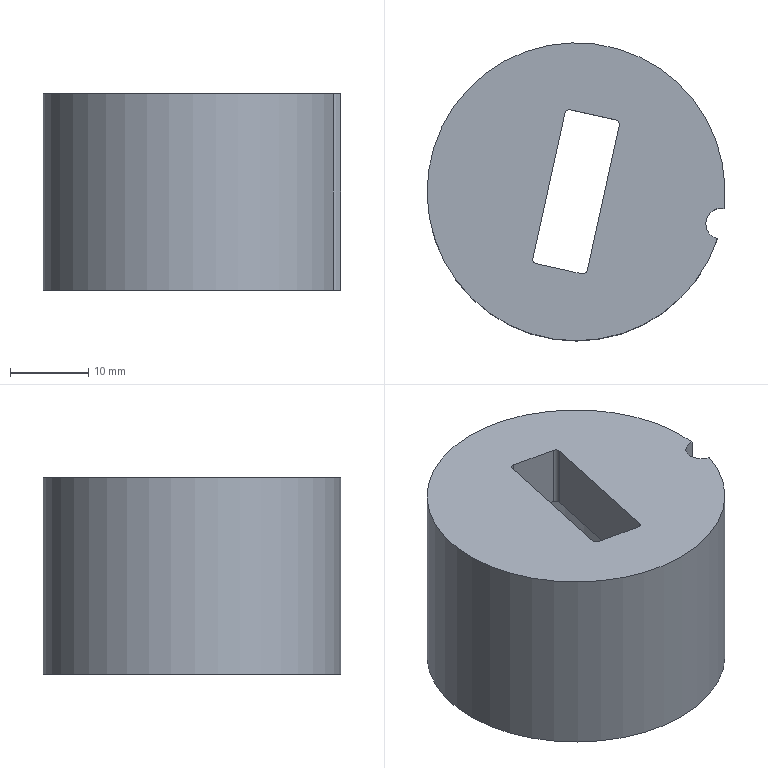Part | NX | features solid 2 | 1 solid | 14 faces | box 38 x 38 x 25 mm | volume 17613 mm3 | cylinder 7 | plane 7 | commonest cylinder face diameters 1.1 x4 4 x1 26.6 x1 38 x1
STEP:
#1=CARTESIAN_POINT('',(36.364,-48.332,31.));
#2=VERTEX_POINT('',#1);
#3=CARTESIAN_POINT('',(36.364,-48.332,56.));
#4=VERTEX_POINT('',#3);
#5=CARTESIAN_POINT('',(36.364,-48.332,43.5));
#6=DIRECTION('',(0.,0.,1.));
#7=VECTOR('',#6,1000.);
#8=LINE('',#5,#7);
#9=EDGE_CURVE('',#2,#4,#8,.T.);
#10=ORIENTED_EDGE('',*,*,#9,.F.);
#11=CARTESIAN_POINT('',(35.507,-52.233,31.));
#12=VERTEX_POINT('',#11);
#13=CARTESIAN_POINT('',(17.482,-46.225,31.));
#14=DIRECTION('',(0.,0.,1.));
#15=DIRECTION('',(0.9767,-0.2148,0.));
#16=AXIS2_PLACEMENT_3D('',#13,#14,#15);
#17=CIRCLE('',#16,19.);
#18=EDGE_CURVE('',#2,#12,#17,.T.);
#19=ORIENTED_EDGE('',*,*,#18,.T.);
#20=CARTESIAN_POINT('',(35.507,-52.233,56.));
#21=VERTEX_POINT('',#20);
#22=CARTESIAN_POINT('',(35.507,-52.233,43.5));
#23=DIRECTION('',(0.,0.,1.));
#24=VECTOR('',#23,1000.);
#25=LINE('',#22,#24);
#26=EDGE_CURVE('',#21,#12,#25,.F.);
#27=ORIENTED_EDGE('',*,*,#26,.F.);
#28=CARTESIAN_POINT('',(17.482,-46.225,56.));
#29=DIRECTION('',(0.,0.,1.));
#30=DIRECTION('',(0.9767,-0.2148,0.));
#31=AXIS2_PLACEMENT_3D('',#28,#29,#30);
#32=CIRCLE('',#31,19.);
#33=EDGE_CURVE('',#4,#21,#32,.T.);
#34=ORIENTED_EDGE('',*,*,#33,.F.);
#35=EDGE_LOOP('',(#10,#19,#27,#34));
#36=FACE_BOUND('',#35,.T.);
#37=CARTESIAN_POINT('',(17.482,-46.225,31.));
#38=DIRECTION('',(0.,0.,1.));
#39=DIRECTION('',(0.9767,-0.2148,0.));
#40=AXIS2_PLACEMENT_3D('',#37,#38,#39);
#41=CYLINDRICAL_SURFACE('',#40,19.);
#42=ADVANCED_FACE('',(#36),#41,.T.);
#43=CARTESIAN_POINT('',(30.471,-49.081,31.));
#44=VERTEX_POINT('',#43);
#45=CARTESIAN_POINT('',(17.482,-46.225,31.));
#46=DIRECTION('',(0.,0.,1.));
#47=DIRECTION('',(0.9767,-0.2148,0.));
#48=AXIS2_PLACEMENT_3D('',#45,#46,#47);
#49=CIRCLE('',#48,13.3);
#50=EDGE_CURVE('',#44,#44,#49,.T.);
#51=ORIENTED_EDGE('',*,*,#50,.T.);
#52=EDGE_LOOP('',(#51));
#53=FACE_BOUND('',#52,.T.);
#54=ORIENTED_EDGE('',*,*,#18,.F.);
#55=CARTESIAN_POINT('',(36.038,-50.305,31.));
#56=DIRECTION('',(0.,0.,1.));
#57=DIRECTION('',(0.9767,-0.2148,0.));
#58=AXIS2_PLACEMENT_3D('',#55,#56,#57);
#59=CIRCLE('',#58,2.);
#60=EDGE_CURVE('',#2,#12,#59,.T.);
#61=ORIENTED_EDGE('',*,*,#60,.T.);
#62=EDGE_LOOP('',(#54,#61));
#63=FACE_BOUND('',#62,.T.);
#64=CARTESIAN_POINT('',(17.482,-46.225,31.));
#65=DIRECTION('',(0.,0.,1.));
#66=DIRECTION('',(0.9767,-0.2148,0.));
#67=AXIS2_PLACEMENT_3D('',#64,#65,#66);
#68=PLANE('',#67);
#69=ADVANCED_FACE('',(#53,#63),#68,.F.);
#70=CARTESIAN_POINT('',(16.055,-36.184,56.));
#71=VERTEX_POINT('',#70);
#72=CARTESIAN_POINT('',(11.974,-54.741,56.));
#73=VERTEX_POINT('',#72);
#74=CARTESIAN_POINT('',(16.173,-35.647,56.));
#75=DIRECTION('',(-0.2148,-0.9767,0.));
#76=VECTOR('',#75,1000.);
#77=LINE('',#74,#76);
#78=EDGE_CURVE('',#71,#73,#77,.T.);
#79=ORIENTED_EDGE('',*,*,#78,.F.);
#80=CARTESIAN_POINT('',(16.71,-35.765,56.));
#81=VERTEX_POINT('',#80);
#82=CARTESIAN_POINT('',(16.592,-36.302,56.));
#83=DIRECTION('',(0.,0.,1.));
#84=DIRECTION('',(0.9767,-0.2148,0.));
#85=AXIS2_PLACEMENT_3D('',#82,#83,#84);
#86=CIRCLE('',#85,0.55);
#87=EDGE_CURVE('',#71,#81,#86,.F.);
#88=ORIENTED_EDGE('',*,*,#87,.T.);
#89=CARTESIAN_POINT('',(22.57,-37.053,56.));
#90=VERTEX_POINT('',#89);
#91=CARTESIAN_POINT('',(23.107,-37.172,56.));
#92=DIRECTION('',(-0.9767,0.2148,0.));
#93=VECTOR('',#92,1000.);
#94=LINE('',#91,#93);
#95=EDGE_CURVE('',#90,#81,#94,.T.);
#96=ORIENTED_EDGE('',*,*,#95,.F.);
#97=CARTESIAN_POINT('',(22.989,-37.709,56.));
#98=VERTEX_POINT('',#97);
#99=CARTESIAN_POINT('',(22.452,-37.591,56.));
#100=DIRECTION('',(0.,0.,1.));
#101=DIRECTION('',(0.9767,-0.2148,0.));
#102=AXIS2_PLACEMENT_3D('',#99,#100,#101);
#103=CIRCLE('',#102,0.55);
#104=EDGE_CURVE('',#90,#98,#103,.F.);
#105=ORIENTED_EDGE('',*,*,#104,.T.);
#106=CARTESIAN_POINT('',(18.909,-56.265,56.));
#107=VERTEX_POINT('',#106);
#108=CARTESIAN_POINT('',(23.107,-37.172,56.));
#109=DIRECTION('',(-0.2148,-0.9767,0.));
#110=VECTOR('',#109,1000.);
#111=LINE('',#108,#110);
#112=EDGE_CURVE('',#98,#107,#111,.T.);
#113=ORIENTED_EDGE('',*,*,#112,.T.);
#114=CARTESIAN_POINT('',(18.253,-56.684,56.));
#115=VERTEX_POINT('',#114);
#116=CARTESIAN_POINT('',(18.371,-56.147,56.));
#117=DIRECTION('',(0.,0.,1.));
#118=DIRECTION('',(0.9767,-0.2148,0.));
#119=AXIS2_PLACEMENT_3D('',#116,#117,#118);
#120=CIRCLE('',#119,0.55);
#121=EDGE_CURVE('',#107,#115,#120,.F.);
#122=ORIENTED_EDGE('',*,*,#121,.T.);
#123=CARTESIAN_POINT('',(12.393,-55.396,56.));
#124=VERTEX_POINT('',#123);
#125=CARTESIAN_POINT('',(11.856,-55.278,56.));
#126=DIRECTION('',(0.9767,-0.2148,0.));
#127=VECTOR('',#126,1000.);
#128=LINE('',#125,#127);
#129=EDGE_CURVE('',#124,#115,#128,.T.);
#130=ORIENTED_EDGE('',*,*,#129,.F.);
#131=CARTESIAN_POINT('',(12.511,-54.859,56.));
#132=DIRECTION('',(0.,0.,1.));
#133=DIRECTION('',(0.9767,-0.2148,0.));
#134=AXIS2_PLACEMENT_3D('',#131,#132,#133);
#135=CIRCLE('',#134,0.55);
#136=EDGE_CURVE('',#124,#73,#135,.F.);
#137=ORIENTED_EDGE('',*,*,#136,.T.);
#138=EDGE_LOOP('',(#79,#88,#96,#105,#113,#122,#130,#137));
#139=FACE_BOUND('',#138,.T.);
#140=CARTESIAN_POINT('',(36.038,-50.305,56.));
#141=DIRECTION('',(0.,0.,1.));
#142=DIRECTION('',(0.9767,-0.2148,0.));
#143=AXIS2_PLACEMENT_3D('',#140,#141,#142);
#144=CIRCLE('',#143,2.);
#145=EDGE_CURVE('',#4,#21,#144,.T.);
#146=ORIENTED_EDGE('',*,*,#145,.F.);
#147=ORIENTED_EDGE('',*,*,#33,.T.);
#148=EDGE_LOOP('',(#146,#147));
#149=FACE_BOUND('',#148,.T.);
#150=CARTESIAN_POINT('',(17.482,-46.225,56.));
#151=DIRECTION('',(0.,0.,1.));
#152=DIRECTION('',(0.9767,-0.2148,0.));
#153=AXIS2_PLACEMENT_3D('',#150,#151,#152);
#154=PLANE('',#153);
#155=ADVANCED_FACE('',(#139,#149),#154,.T.);
#156=ORIENTED_EDGE('',*,*,#50,.F.);
#157=EDGE_LOOP('',(#156));
#158=FACE_BOUND('',#157,.T.);
#159=CARTESIAN_POINT('',(30.471,-49.081,48.));
#160=VERTEX_POINT('',#159);
#161=CARTESIAN_POINT('',(17.482,-46.225,48.));
#162=DIRECTION('',(0.,0.,1.));
#163=DIRECTION('',(0.9767,-0.2148,0.));
#164=AXIS2_PLACEMENT_3D('',#161,#162,#163);
#165=CIRCLE('',#164,13.3);
#166=EDGE_CURVE('',#160,#160,#165,.T.);
#167=ORIENTED_EDGE('',*,*,#166,.T.);
#168=EDGE_LOOP('',(#167));
#169=FACE_BOUND('',#168,.T.);
#170=CARTESIAN_POINT('',(17.482,-46.225,31.));
#171=DIRECTION('',(0.,0.,1.));
#172=DIRECTION('',(0.9767,-0.2148,0.));
#173=AXIS2_PLACEMENT_3D('',#170,#171,#172);
#174=CYLINDRICAL_SURFACE('',#173,13.3);
#175=ADVANCED_FACE('',(#158,#169),#174,.F.);
#176=CARTESIAN_POINT('',(22.989,-37.709,48.));
#177=VERTEX_POINT('',#176);
#178=CARTESIAN_POINT('',(18.909,-56.265,48.));
#179=VERTEX_POINT('',#178);
#180=CARTESIAN_POINT('',(20.949,-46.987,48.));
#181=DIRECTION('',(-0.2148,-0.9767,0.));
#182=VECTOR('',#181,1000.);
#183=LINE('',#180,#182);
#184=EDGE_CURVE('',#177,#179,#183,.T.);
#185=ORIENTED_EDGE('',*,*,#184,.F.);
#186=CARTESIAN_POINT('',(22.57,-37.053,48.));
#187=VERTEX_POINT('',#186);
#188=CARTESIAN_POINT('',(22.452,-37.591,48.));
#189=DIRECTION('',(0.,0.,1.));
#190=DIRECTION('',(0.9767,-0.2148,0.));
#191=AXIS2_PLACEMENT_3D('',#188,#189,#190);
#192=CIRCLE('',#191,0.55);
#193=EDGE_CURVE('',#177,#187,#192,.T.);
#194=ORIENTED_EDGE('',*,*,#193,.T.);
#195=CARTESIAN_POINT('',(16.71,-35.765,48.));
#196=VERTEX_POINT('',#195);
#197=CARTESIAN_POINT('',(19.64,-36.409,48.));
#198=DIRECTION('',(-0.9767,0.2148,0.));
#199=VECTOR('',#198,1000.);
#200=LINE('',#197,#199);
#201=EDGE_CURVE('',#187,#196,#200,.T.);
#202=ORIENTED_EDGE('',*,*,#201,.T.);
#203=CARTESIAN_POINT('',(16.055,-36.184,48.));
#204=VERTEX_POINT('',#203);
#205=CARTESIAN_POINT('',(16.592,-36.302,48.));
#206=DIRECTION('',(0.,0.,1.));
#207=DIRECTION('',(0.9767,-0.2148,0.));
#208=AXIS2_PLACEMENT_3D('',#205,#206,#207);
#209=CIRCLE('',#208,0.55);
#210=EDGE_CURVE('',#196,#204,#209,.T.);
#211=ORIENTED_EDGE('',*,*,#210,.T.);
#212=CARTESIAN_POINT('',(11.974,-54.741,48.));
#213=VERTEX_POINT('',#212);
#214=CARTESIAN_POINT('',(14.014,-45.462,48.));
#215=DIRECTION('',(-0.2148,-0.9767,0.));
#216=VECTOR('',#215,1000.);
#217=LINE('',#214,#216);
#218=EDGE_CURVE('',#204,#213,#217,.T.);
#219=ORIENTED_EDGE('',*,*,#218,.T.);
#220=CARTESIAN_POINT('',(12.393,-55.396,48.));
#221=VERTEX_POINT('',#220);
#222=CARTESIAN_POINT('',(12.511,-54.859,48.));
#223=DIRECTION('',(0.,0.,1.));
#224=DIRECTION('',(0.9767,-0.2148,0.));
#225=AXIS2_PLACEMENT_3D('',#222,#223,#224);
#226=CIRCLE('',#225,0.55);
#227=EDGE_CURVE('',#213,#221,#226,.T.);
#228=ORIENTED_EDGE('',*,*,#227,.T.);
#229=CARTESIAN_POINT('',(18.253,-56.684,48.));
#230=VERTEX_POINT('',#229);
#231=CARTESIAN_POINT('',(15.323,-56.04,48.));
#232=DIRECTION('',(0.9767,-0.2148,0.));
#233=VECTOR('',#232,1000.);
#234=LINE('',#231,#233);
#235=EDGE_CURVE('',#221,#230,#234,.T.);
#236=ORIENTED_EDGE('',*,*,#235,.T.);
#237=CARTESIAN_POINT('',(18.371,-56.147,48.));
#238=DIRECTION('',(0.,0.,1.));
#239=DIRECTION('',(0.9767,-0.2148,0.));
#240=AXIS2_PLACEMENT_3D('',#237,#238,#239);
#241=CIRCLE('',#240,0.55);
#242=EDGE_CURVE('',#230,#179,#241,.T.);
#243=ORIENTED_EDGE('',*,*,#242,.T.);
#244=EDGE_LOOP('',(#185,#194,#202,#211,#219,#228,#236,#243));
#245=FACE_BOUND('',#244,.T.);
#246=ORIENTED_EDGE('',*,*,#166,.F.);
#247=EDGE_LOOP('',(#246));
#248=FACE_BOUND('',#247,.T.);
#249=CARTESIAN_POINT('',(17.482,-46.225,48.));
#250=DIRECTION('',(0.,0.,1.));
#251=DIRECTION('',(0.9767,-0.2148,0.));
#252=AXIS2_PLACEMENT_3D('',#249,#250,#251);
#253=PLANE('',#252);
#254=ADVANCED_FACE('',(#245,#248),#253,.F.);
#255=ORIENTED_EDGE('',*,*,#9,.T.);
#256=ORIENTED_EDGE('',*,*,#145,.T.);
#257=ORIENTED_EDGE('',*,*,#26,.T.);
#258=ORIENTED_EDGE('',*,*,#60,.F.);
#259=EDGE_LOOP('',(#255,#256,#257,#258));
#260=FACE_BOUND('',#259,.T.);
#261=CARTESIAN_POINT('',(36.038,-50.305,31.));
#262=DIRECTION('',(0.,0.,1.));
#263=DIRECTION('',(0.9767,-0.2148,0.));
#264=AXIS2_PLACEMENT_3D('',#261,#262,#263);
#265=CYLINDRICAL_SURFACE('',#264,2.);
#266=ADVANCED_FACE('',(#260),#265,.F.);
#267=ORIENTED_EDGE('',*,*,#78,.T.);
#268=CARTESIAN_POINT('',(11.974,-54.741,48.));
#269=DIRECTION('',(0.,0.,1.));
#270=VECTOR('',#269,1000.);
#271=LINE('',#268,#270);
#272=EDGE_CURVE('',#73,#213,#271,.F.);
#273=ORIENTED_EDGE('',*,*,#272,.T.);
#274=ORIENTED_EDGE('',*,*,#218,.F.);
#275=CARTESIAN_POINT('',(16.055,-36.184,56.));
#276=DIRECTION('',(0.,0.,1.));
#277=VECTOR('',#276,1000.);
#278=LINE('',#275,#277);
#279=EDGE_CURVE('',#204,#71,#278,.T.);
#280=ORIENTED_EDGE('',*,*,#279,.T.);
#281=EDGE_LOOP('',(#267,#273,#274,#280));
#282=FACE_BOUND('',#281,.T.);
#283=CARTESIAN_POINT('',(16.173,-35.647,31.));
#284=DIRECTION('',(-0.9767,0.2148,0.));
#285=DIRECTION('',(0.,0.,1.));
#286=AXIS2_PLACEMENT_3D('',#283,#284,#285);
#287=PLANE('',#286);
#288=ADVANCED_FACE('',(#282),#287,.F.);
#289=ORIENTED_EDGE('',*,*,#129,.T.);
#290=CARTESIAN_POINT('',(18.253,-56.684,31.));
#291=DIRECTION('',(0.,0.,1.));
#292=VECTOR('',#291,1000.);
#293=LINE('',#290,#292);
#294=EDGE_CURVE('',#115,#230,#293,.F.);
#295=ORIENTED_EDGE('',*,*,#294,.T.);
#296=ORIENTED_EDGE('',*,*,#235,.F.);
#297=CARTESIAN_POINT('',(12.393,-55.396,56.));
#298=DIRECTION('',(0.,0.,1.));
#299=VECTOR('',#298,1000.);
#300=LINE('',#297,#299);
#301=EDGE_CURVE('',#221,#124,#300,.T.);
#302=ORIENTED_EDGE('',*,*,#301,.T.);
#303=EDGE_LOOP('',(#289,#295,#296,#302));
#304=FACE_BOUND('',#303,.T.);
#305=CARTESIAN_POINT('',(11.856,-55.278,31.));
#306=DIRECTION('',(-0.2148,-0.9767,0.));
#307=DIRECTION('',(0.,0.,-1.));
#308=AXIS2_PLACEMENT_3D('',#305,#306,#307);
#309=PLANE('',#308);
#310=ADVANCED_FACE('',(#304),#309,.F.);
#311=ORIENTED_EDGE('',*,*,#112,.F.);
#312=CARTESIAN_POINT('',(22.989,-37.709,31.));
#313=DIRECTION('',(0.,0.,1.));
#314=VECTOR('',#313,1000.);
#315=LINE('',#312,#314);
#316=EDGE_CURVE('',#98,#177,#315,.F.);
#317=ORIENTED_EDGE('',*,*,#316,.T.);
#318=ORIENTED_EDGE('',*,*,#184,.T.);
#319=CARTESIAN_POINT('',(18.909,-56.265,31.));
#320=DIRECTION('',(0.,0.,1.));
#321=VECTOR('',#320,1000.);
#322=LINE('',#319,#321);
#323=EDGE_CURVE('',#179,#107,#322,.T.);
#324=ORIENTED_EDGE('',*,*,#323,.T.);
#325=EDGE_LOOP('',(#311,#317,#318,#324));
#326=FACE_BOUND('',#325,.T.);
#327=CARTESIAN_POINT('',(23.107,-37.172,31.));
#328=DIRECTION('',(-0.9767,0.2148,0.));
#329=DIRECTION('',(0.,0.,1.));
#330=AXIS2_PLACEMENT_3D('',#327,#328,#329);
#331=PLANE('',#330);
#332=ADVANCED_FACE('',(#326),#331,.T.);
#333=ORIENTED_EDGE('',*,*,#201,.F.);
#334=CARTESIAN_POINT('',(22.57,-37.053,31.));
#335=DIRECTION('',(0.,0.,1.));
#336=VECTOR('',#335,1000.);
#337=LINE('',#334,#336);
#338=EDGE_CURVE('',#187,#90,#337,.T.);
#339=ORIENTED_EDGE('',*,*,#338,.T.);
#340=ORIENTED_EDGE('',*,*,#95,.T.);
#341=CARTESIAN_POINT('',(16.71,-35.765,48.));
#342=DIRECTION('',(0.,0.,1.));
#343=VECTOR('',#342,1000.);
#344=LINE('',#341,#343);
#345=EDGE_CURVE('',#81,#196,#344,.F.);
#346=ORIENTED_EDGE('',*,*,#345,.T.);
#347=EDGE_LOOP('',(#333,#339,#340,#346));
#348=FACE_BOUND('',#347,.T.);
#349=CARTESIAN_POINT('',(23.107,-37.172,31.));
#350=DIRECTION('',(0.2148,0.9767,0.));
#351=DIRECTION('',(0.,0.,1.));
#352=AXIS2_PLACEMENT_3D('',#349,#350,#351);
#353=PLANE('',#352);
#354=ADVANCED_FACE('',(#348),#353,.F.);
#355=ORIENTED_EDGE('',*,*,#193,.F.);
#356=ORIENTED_EDGE('',*,*,#316,.F.);
#357=ORIENTED_EDGE('',*,*,#104,.F.);
#358=ORIENTED_EDGE('',*,*,#338,.F.);
#359=EDGE_LOOP('',(#355,#356,#357,#358));
#360=FACE_BOUND('',#359,.T.);
#361=CARTESIAN_POINT('',(22.452,-37.591,31.));
#362=DIRECTION('',(0.,0.,1.));
#363=DIRECTION('',(0.9767,-0.2148,0.));
#364=AXIS2_PLACEMENT_3D('',#361,#362,#363);
#365=CYLINDRICAL_SURFACE('',#364,0.55);
#366=ADVANCED_FACE('',(#360),#365,.F.);
#367=ORIENTED_EDGE('',*,*,#242,.F.);
#368=ORIENTED_EDGE('',*,*,#294,.F.);
#369=ORIENTED_EDGE('',*,*,#121,.F.);
#370=ORIENTED_EDGE('',*,*,#323,.F.);
#371=EDGE_LOOP('',(#367,#368,#369,#370));
#372=FACE_BOUND('',#371,.T.);
#373=CARTESIAN_POINT('',(18.371,-56.147,31.));
#374=DIRECTION('',(0.,0.,1.));
#375=DIRECTION('',(0.9767,-0.2148,0.));
#376=AXIS2_PLACEMENT_3D('',#373,#374,#375);
#377=CYLINDRICAL_SURFACE('',#376,0.55);
#378=ADVANCED_FACE('',(#372),#377,.F.);
#379=ORIENTED_EDGE('',*,*,#227,.F.);
#380=ORIENTED_EDGE('',*,*,#272,.F.);
#381=ORIENTED_EDGE('',*,*,#136,.F.);
#382=ORIENTED_EDGE('',*,*,#301,.F.);
#383=EDGE_LOOP('',(#379,#380,#381,#382));
#384=FACE_BOUND('',#383,.T.);
#385=CARTESIAN_POINT('',(12.511,-54.859,31.));
#386=DIRECTION('',(0.,0.,-1.));
#387=DIRECTION('',(-0.9767,0.2148,0.));
#388=AXIS2_PLACEMENT_3D('',#385,#386,#387);
#389=CYLINDRICAL_SURFACE('',#388,0.55);
#390=ADVANCED_FACE('',(#384),#389,.F.);
#391=ORIENTED_EDGE('',*,*,#210,.F.);
#392=ORIENTED_EDGE('',*,*,#345,.F.);
#393=ORIENTED_EDGE('',*,*,#87,.F.);
#394=ORIENTED_EDGE('',*,*,#279,.F.);
#395=EDGE_LOOP('',(#391,#392,#393,#394));
#396=FACE_BOUND('',#395,.T.);
#397=CARTESIAN_POINT('',(16.592,-36.302,31.));
#398=DIRECTION('',(0.,0.,-1.));
#399=DIRECTION('',(-0.9767,0.2148,0.));
#400=AXIS2_PLACEMENT_3D('',#397,#398,#399);
#401=CYLINDRICAL_SURFACE('',#400,0.55);
#402=ADVANCED_FACE('',(#396),#401,.F.);
#403=CLOSED_SHELL('',(#42,#69,#155,#175,#254,#266,#288,#310,#332,#354,#366,#378,#390,#402));
#404=MANIFOLD_SOLID_BREP('',#403);
#405=(LENGTH_UNIT()NAMED_UNIT(*)SI_UNIT(.MILLI.,.METRE.));
#406=UNCERTAINTY_MEASURE_WITH_UNIT(LENGTH_MEASURE(0.00001),#405,'','');
#407=(NAMED_UNIT(*)PLANE_ANGLE_UNIT()SI_UNIT($,.RADIAN.));
#408=(NAMED_UNIT(*)SI_UNIT($,.STERADIAN.)SOLID_ANGLE_UNIT());
#409=(GEOMETRIC_REPRESENTATION_CONTEXT(3)GLOBAL_UNCERTAINTY_ASSIGNED_CONTEXT((#406))GLOBAL_UNIT_ASSIGNED_CONTEXT((#405,#407,#408))REPRESENTATION_CONTEXT('',''));
#410=ADVANCED_BREP_SHAPE_REPRESENTATION('',(#404),#409);